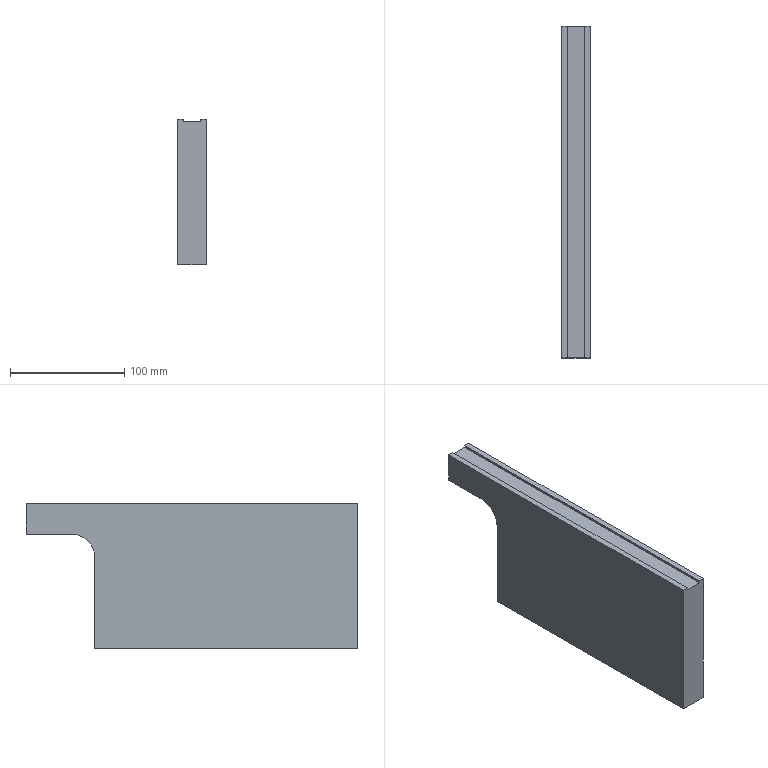Part | STEP file | Tube necking machine_id718_x_t | 1 solid | 13 faces | box 25 x 290 x 127 mm | volume 764196 mm3 | plane 12 | cylinder 1 | commonest cylinder face diameters 40 x1
STEP:
#1=CARTESIAN_POINT('',(0.,0.,0.));
#2=DIRECTION('',(0.,0.,1.));
#3=DIRECTION('',(1.,0.,0.));
#4=AXIS2_PLACEMENT_3D('',#1,#2,#3);
#5=CARTESIAN_POINT('',(192.5,-276.,145.));
#6=VERTEX_POINT('',#5);
#7=CARTESIAN_POINT('',(192.5,-276.,147.));
#8=VERTEX_POINT('',#7);
#9=CARTESIAN_POINT('',(192.5,-276.,146.181));
#10=DIRECTION('',(0.,0.,1.));
#11=VECTOR('',#10,1.);
#12=LINE('',#9,#11);
#13=CARTESIAN_POINT('',(197.5,-276.,110.));
#14=DIRECTION('',(0.,1.,0.));
#15=DIRECTION('',(0.,0.,1.));
#16=AXIS2_PLACEMENT_3D('',#13,#14,#15);
#17=PLANE('',#16);
#18=CARTESIAN_POINT('',(36.181,-5.));
#19=DIRECTION('',(1.,0.));
#20=VECTOR('',#19,1.);
#21=LINE('',#18,#20);
#22=(GEOMETRIC_REPRESENTATION_CONTEXT(2)PARAMETRIC_REPRESENTATION_CONTEXT()REPRESENTATION_CONTEXT('',''));
#23=DEFINITIONAL_REPRESENTATION('',(#21),#22);
#24=PCURVE('',#17,#23);
#25=CARTESIAN_POINT('',(192.5,795.73,146.181));
#26=DIRECTION('',(1.,0.,0.));
#27=DIRECTION('',(0.,0.,1.));
#28=AXIS2_PLACEMENT_3D('',#25,#26,#27);
#29=PLANE('',#28);
#30=CARTESIAN_POINT('',(0.,1071.73));
#31=DIRECTION('',(1.,0.));
#32=VECTOR('',#31,1.);
#33=LINE('',#30,#32);
#34=(GEOMETRIC_REPRESENTATION_CONTEXT(2)PARAMETRIC_REPRESENTATION_CONTEXT()REPRESENTATION_CONTEXT('',''));
#35=DEFINITIONAL_REPRESENTATION('',(#33),#34);
#36=PCURVE('',#29,#35);
#37=SURFACE_CURVE('',#12,(#24,#36),.PCURVE_S1.);
#38=EDGE_CURVE('',#6,#8,#37,.T.);
#39=ORIENTED_EDGE('',*,*,#38,.F.);
#40=CARTESIAN_POINT('',(177.5,-276.,145.));
#41=VERTEX_POINT('',#40);
#42=CARTESIAN_POINT('',(192.5,-276.,145.));
#43=DIRECTION('',(1.,0.,0.));
#44=VECTOR('',#43,1.);
#45=LINE('',#42,#44);
#46=CARTESIAN_POINT('',(35.,-5.));
#47=DIRECTION('',(0.,1.));
#48=VECTOR('',#47,1.);
#49=LINE('',#46,#48);
#50=(GEOMETRIC_REPRESENTATION_CONTEXT(2)PARAMETRIC_REPRESENTATION_CONTEXT()REPRESENTATION_CONTEXT('',''));
#51=DEFINITIONAL_REPRESENTATION('',(#49),#50);
#52=PCURVE('',#17,#51);
#53=CARTESIAN_POINT('',(192.5,795.73,145.));
#54=DIRECTION('',(0.,0.,-1.));
#55=DIRECTION('',(0.,-1.,0.));
#56=AXIS2_PLACEMENT_3D('',#53,#54,#55);
#57=PLANE('',#56);
#58=CARTESIAN_POINT('',(1071.73,0.));
#59=DIRECTION('',(0.,-1.));
#60=VECTOR('',#59,1.);
#61=LINE('',#58,#60);
#62=(GEOMETRIC_REPRESENTATION_CONTEXT(2)PARAMETRIC_REPRESENTATION_CONTEXT()REPRESENTATION_CONTEXT('',''));
#63=DEFINITIONAL_REPRESENTATION('',(#61),#62);
#64=PCURVE('',#57,#63);
#65=SURFACE_CURVE('',#45,(#52,#64),.PCURVE_S1.);
#66=EDGE_CURVE('',#41,#6,#65,.T.);
#67=ORIENTED_EDGE('',*,*,#66,.F.);
#68=CARTESIAN_POINT('',(177.5,-276.,147.));
#69=VERTEX_POINT('',#68);
#70=CARTESIAN_POINT('',(177.5,-276.,145.));
#71=DIRECTION('',(0.,0.,-1.));
#72=VECTOR('',#71,1.);
#73=LINE('',#70,#72);
#74=CARTESIAN_POINT('',(35.,-20.));
#75=DIRECTION('',(-1.,0.));
#76=VECTOR('',#75,1.);
#77=LINE('',#74,#76);
#78=(GEOMETRIC_REPRESENTATION_CONTEXT(2)PARAMETRIC_REPRESENTATION_CONTEXT()REPRESENTATION_CONTEXT('',''));
#79=DEFINITIONAL_REPRESENTATION('',(#77),#78);
#80=PCURVE('',#17,#79);
#81=CARTESIAN_POINT('',(177.5,795.73,145.));
#82=DIRECTION('',(-1.,0.,0.));
#83=DIRECTION('',(0.,0.,-1.));
#84=AXIS2_PLACEMENT_3D('',#81,#82,#83);
#85=PLANE('',#84);
#86=CARTESIAN_POINT('',(0.,1071.73));
#87=DIRECTION('',(1.,0.));
#88=VECTOR('',#87,1.);
#89=LINE('',#86,#88);
#90=(GEOMETRIC_REPRESENTATION_CONTEXT(2)PARAMETRIC_REPRESENTATION_CONTEXT()REPRESENTATION_CONTEXT('',''));
#91=DEFINITIONAL_REPRESENTATION('',(#89),#90);
#92=PCURVE('',#85,#91);
#93=SURFACE_CURVE('',#73,(#80,#92),.PCURVE_S1.);
#94=EDGE_CURVE('',#69,#41,#93,.T.);
#95=ORIENTED_EDGE('',*,*,#94,.F.);
#96=CARTESIAN_POINT('',(172.5,-276.,147.));
#97=VERTEX_POINT('',#96);
#98=CARTESIAN_POINT('',(197.5,-276.,147.));
#99=DIRECTION('',(1.,0.,0.));
#100=VECTOR('',#99,1.);
#101=LINE('',#98,#100);
#102=CARTESIAN_POINT('',(37.,0.));
#103=DIRECTION('',(0.,1.));
#104=VECTOR('',#103,1.);
#105=LINE('',#102,#104);
#106=(GEOMETRIC_REPRESENTATION_CONTEXT(2)PARAMETRIC_REPRESENTATION_CONTEXT()REPRESENTATION_CONTEXT('',''));
#107=DEFINITIONAL_REPRESENTATION('',(#105),#106);
#108=PCURVE('',#17,#107);
#109=CARTESIAN_POINT('',(0.,0.,147.));
#110=DIRECTION('',(0.,0.,1.));
#111=DIRECTION('',(-1.,0.,0.));
#112=AXIS2_PLACEMENT_3D('',#109,#110,#111);
#113=PLANE('',#112);
#114=CARTESIAN_POINT('',(-197.5,276.));
#115=DIRECTION('',(-1.,0.));
#116=VECTOR('',#115,1.);
#117=LINE('',#114,#116);
#118=(GEOMETRIC_REPRESENTATION_CONTEXT(2)PARAMETRIC_REPRESENTATION_CONTEXT()REPRESENTATION_CONTEXT('',''));
#119=DEFINITIONAL_REPRESENTATION('',(#117),#118);
#120=PCURVE('',#113,#119);
#121=SURFACE_CURVE('',#101,(#108,#120),.PCURVE_S1.);
#122=EDGE_CURVE('',#97,#69,#121,.T.);
#123=ORIENTED_EDGE('',*,*,#122,.F.);
#124=CARTESIAN_POINT('',(172.5,-276.,20.));
#125=VERTEX_POINT('',#124);
#126=CARTESIAN_POINT('',(172.5,-276.,110.));
#127=DIRECTION('',(0.,0.,1.));
#128=VECTOR('',#127,1.);
#129=LINE('',#126,#128);
#130=CARTESIAN_POINT('',(0.,-25.));
#131=DIRECTION('',(1.,0.));
#132=VECTOR('',#131,1.);
#133=LINE('',#130,#132);
#134=(GEOMETRIC_REPRESENTATION_CONTEXT(2)PARAMETRIC_REPRESENTATION_CONTEXT()REPRESENTATION_CONTEXT('',''));
#135=DEFINITIONAL_REPRESENTATION('',(#133),#134);
#136=PCURVE('',#17,#135);
#137=CARTESIAN_POINT('',(172.5,-276.,110.));
#138=DIRECTION('',(1.,0.,0.));
#139=DIRECTION('',(0.,0.,1.));
#140=AXIS2_PLACEMENT_3D('',#137,#138,#139);
#141=PLANE('',#140);
#142=CARTESIAN_POINT('',(0.,0.));
#143=DIRECTION('',(1.,0.));
#144=VECTOR('',#143,1.);
#145=LINE('',#142,#144);
#146=(GEOMETRIC_REPRESENTATION_CONTEXT(2)PARAMETRIC_REPRESENTATION_CONTEXT()REPRESENTATION_CONTEXT('',''));
#147=DEFINITIONAL_REPRESENTATION('',(#145),#146);
#148=PCURVE('',#141,#147);
#149=SURFACE_CURVE('',#129,(#136,#148),.PCURVE_S1.);
#150=EDGE_CURVE('',#125,#97,#149,.T.);
#151=ORIENTED_EDGE('',*,*,#150,.F.);
#152=CARTESIAN_POINT('',(197.5,-276.,20.));
#153=VERTEX_POINT('',#152);
#154=CARTESIAN_POINT('',(197.5,-276.,20.));
#155=DIRECTION('',(1.,0.,0.));
#156=VECTOR('',#155,1.);
#157=LINE('',#154,#156);
#158=CARTESIAN_POINT('',(-90.,0.));
#159=DIRECTION('',(0.,1.));
#160=VECTOR('',#159,1.);
#161=LINE('',#158,#160);
#162=(GEOMETRIC_REPRESENTATION_CONTEXT(2)PARAMETRIC_REPRESENTATION_CONTEXT()REPRESENTATION_CONTEXT('',''));
#163=DEFINITIONAL_REPRESENTATION('',(#161),#162);
#164=PCURVE('',#17,#163);
#165=CARTESIAN_POINT('',(0.,0.,20.));
#166=DIRECTION('',(0.,0.,1.));
#167=DIRECTION('',(-1.,0.,0.));
#168=AXIS2_PLACEMENT_3D('',#165,#166,#167);
#169=PLANE('',#168);
#170=CARTESIAN_POINT('',(-197.5,276.));
#171=DIRECTION('',(-1.,0.));
#172=VECTOR('',#171,1.);
#173=LINE('',#170,#172);
#174=(GEOMETRIC_REPRESENTATION_CONTEXT(2)PARAMETRIC_REPRESENTATION_CONTEXT()REPRESENTATION_CONTEXT('',''));
#175=DEFINITIONAL_REPRESENTATION('',(#173),#174);
#176=PCURVE('',#169,#175);
#177=SURFACE_CURVE('',#157,(#164,#176),.PCURVE_S1.);
#178=EDGE_CURVE('',#125,#153,#177,.T.);
#179=ORIENTED_EDGE('',*,*,#178,.T.);
#180=CARTESIAN_POINT('',(197.5,-276.,147.));
#181=VERTEX_POINT('',#180);
#182=CARTESIAN_POINT('',(197.5,-276.,110.));
#183=DIRECTION('',(0.,0.,1.));
#184=VECTOR('',#183,1.);
#185=LINE('',#182,#184);
#186=CARTESIAN_POINT('',(0.,0.));
#187=DIRECTION('',(1.,0.));
#188=VECTOR('',#187,1.);
#189=LINE('',#186,#188);
#190=(GEOMETRIC_REPRESENTATION_CONTEXT(2)PARAMETRIC_REPRESENTATION_CONTEXT()REPRESENTATION_CONTEXT('',''));
#191=DEFINITIONAL_REPRESENTATION('',(#189),#190);
#192=PCURVE('',#17,#191);
#193=CARTESIAN_POINT('',(197.5,-46.,110.));
#194=DIRECTION('',(-1.,0.,0.));
#195=DIRECTION('',(0.,0.,-1.));
#196=AXIS2_PLACEMENT_3D('',#193,#194,#195);
#197=PLANE('',#196);
#198=CARTESIAN_POINT('',(0.,230.));
#199=DIRECTION('',(-1.,0.));
#200=VECTOR('',#199,1.);
#201=LINE('',#198,#200);
#202=(GEOMETRIC_REPRESENTATION_CONTEXT(2)PARAMETRIC_REPRESENTATION_CONTEXT()REPRESENTATION_CONTEXT('',''));
#203=DEFINITIONAL_REPRESENTATION('',(#201),#202);
#204=PCURVE('',#197,#203);
#205=SURFACE_CURVE('',#185,(#192,#204),.PCURVE_S1.);
#206=EDGE_CURVE('',#153,#181,#205,.T.);
#207=ORIENTED_EDGE('',*,*,#206,.T.);
#208=CARTESIAN_POINT('',(197.5,-276.,147.));
#209=DIRECTION('',(1.,0.,0.));
#210=VECTOR('',#209,1.);
#211=LINE('',#208,#210);
#212=CARTESIAN_POINT('',(37.,0.));
#213=DIRECTION('',(0.,1.));
#214=VECTOR('',#213,1.);
#215=LINE('',#212,#214);
#216=(GEOMETRIC_REPRESENTATION_CONTEXT(2)PARAMETRIC_REPRESENTATION_CONTEXT()REPRESENTATION_CONTEXT('',''));
#217=DEFINITIONAL_REPRESENTATION('',(#215),#216);
#218=PCURVE('',#17,#217);
#219=CARTESIAN_POINT('',(0.,0.,147.));
#220=DIRECTION('',(0.,0.,1.));
#221=DIRECTION('',(-1.,0.,0.));
#222=AXIS2_PLACEMENT_3D('',#219,#220,#221);
#223=PLANE('',#222);
#224=CARTESIAN_POINT('',(-197.5,276.));
#225=DIRECTION('',(-1.,0.));
#226=VECTOR('',#225,1.);
#227=LINE('',#224,#226);
#228=(GEOMETRIC_REPRESENTATION_CONTEXT(2)PARAMETRIC_REPRESENTATION_CONTEXT()REPRESENTATION_CONTEXT('',''));
#229=DEFINITIONAL_REPRESENTATION('',(#227),#228);
#230=PCURVE('',#223,#229);
#231=SURFACE_CURVE('',#211,(#218,#230),.PCURVE_S1.);
#232=EDGE_CURVE('',#8,#181,#231,.T.);
#233=ORIENTED_EDGE('',*,*,#232,.F.);
#234=EDGE_LOOP('',(#39,#67,#95,#123,#151,#179,#207,#233));
#235=FACE_BOUND('',#234,.T.);
#236=ADVANCED_FACE('',(#235),#17,.F.);
#237=CARTESIAN_POINT('',(177.5,14.,147.));
#238=VERTEX_POINT('',#237);
#239=CARTESIAN_POINT('',(177.5,0.,147.));
#240=DIRECTION('',(0.,-1.,0.));
#241=VECTOR('',#240,1.);
#242=LINE('',#239,#241);
#243=CARTESIAN_POINT('',(-177.5,0.));
#244=DIRECTION('',(0.,1.));
#245=VECTOR('',#244,1.);
#246=LINE('',#243,#245);
#247=(GEOMETRIC_REPRESENTATION_CONTEXT(2)PARAMETRIC_REPRESENTATION_CONTEXT()REPRESENTATION_CONTEXT('',''));
#248=DEFINITIONAL_REPRESENTATION('',(#246),#247);
#249=PCURVE('',#113,#248);
#250=CARTESIAN_POINT('',(-2.,795.73));
#251=DIRECTION('',(0.,1.));
#252=VECTOR('',#251,1.);
#253=LINE('',#250,#252);
#254=(GEOMETRIC_REPRESENTATION_CONTEXT(2)PARAMETRIC_REPRESENTATION_CONTEXT()REPRESENTATION_CONTEXT('',''));
#255=DEFINITIONAL_REPRESENTATION('',(#253),#254);
#256=PCURVE('',#85,#255);
#257=SURFACE_CURVE('',#242,(#249,#256),.PCURVE_S1.);
#258=EDGE_CURVE('',#238,#69,#257,.T.);
#259=ORIENTED_EDGE('',*,*,#258,.F.);
#260=CARTESIAN_POINT('',(172.5,14.,147.));
#261=VERTEX_POINT('',#260);
#262=CARTESIAN_POINT('',(197.5,14.,147.));
#263=DIRECTION('',(1.,0.,0.));
#264=VECTOR('',#263,1.);
#265=LINE('',#262,#264);
#266=CARTESIAN_POINT('',(-197.5,-14.));
#267=DIRECTION('',(-1.,0.));
#268=VECTOR('',#267,1.);
#269=LINE('',#266,#268);
#270=(GEOMETRIC_REPRESENTATION_CONTEXT(2)PARAMETRIC_REPRESENTATION_CONTEXT()REPRESENTATION_CONTEXT('',''));
#271=DEFINITIONAL_REPRESENTATION('',(#269),#270);
#272=PCURVE('',#113,#271);
#273=CARTESIAN_POINT('',(197.5,14.,151.));
#274=DIRECTION('',(0.,1.,0.));
#275=DIRECTION('',(-1.,0.,0.));
#276=AXIS2_PLACEMENT_3D('',#273,#274,#275);
#277=PLANE('',#276);
#278=CARTESIAN_POINT('',(0.,-4.));
#279=DIRECTION('',(-1.,0.));
#280=VECTOR('',#279,1.);
#281=LINE('',#278,#280);
#282=(GEOMETRIC_REPRESENTATION_CONTEXT(2)PARAMETRIC_REPRESENTATION_CONTEXT()REPRESENTATION_CONTEXT('',''));
#283=DEFINITIONAL_REPRESENTATION('',(#281),#282);
#284=PCURVE('',#277,#283);
#285=SURFACE_CURVE('',#265,(#272,#284),.PCURVE_S1.);
#286=EDGE_CURVE('',#261,#238,#285,.T.);
#287=ORIENTED_EDGE('',*,*,#286,.F.);
#288=CARTESIAN_POINT('',(172.5,-276.,147.));
#289=DIRECTION('',(0.,-1.,0.));
#290=VECTOR('',#289,1.);
#291=LINE('',#288,#290);
#292=CARTESIAN_POINT('',(-172.5,276.));
#293=DIRECTION('',(0.,1.));
#294=VECTOR('',#293,1.);
#295=LINE('',#292,#294);
#296=(GEOMETRIC_REPRESENTATION_CONTEXT(2)PARAMETRIC_REPRESENTATION_CONTEXT()REPRESENTATION_CONTEXT('',''));
#297=DEFINITIONAL_REPRESENTATION('',(#295),#296);
#298=PCURVE('',#113,#297);
#299=CARTESIAN_POINT('',(37.,0.));
#300=DIRECTION('',(0.,1.));
#301=VECTOR('',#300,1.);
#302=LINE('',#299,#301);
#303=(GEOMETRIC_REPRESENTATION_CONTEXT(2)PARAMETRIC_REPRESENTATION_CONTEXT()REPRESENTATION_CONTEXT('',''));
#304=DEFINITIONAL_REPRESENTATION('',(#302),#303);
#305=PCURVE('',#141,#304);
#306=SURFACE_CURVE('',#291,(#298,#305),.PCURVE_S1.);
#307=EDGE_CURVE('',#261,#97,#306,.T.);
#308=ORIENTED_EDGE('',*,*,#307,.T.);
#309=ORIENTED_EDGE('',*,*,#122,.T.);
#310=EDGE_LOOP('',(#259,#287,#308,#309));
#311=FACE_BOUND('',#310,.T.);
#312=ADVANCED_FACE('',(#311),#113,.T.);
#313=ORIENTED_EDGE('',*,*,#206,.F.);
#314=CARTESIAN_POINT('',(197.5,-46.,20.));
#315=VERTEX_POINT('',#314);
#316=CARTESIAN_POINT('',(197.5,-46.,20.));
#317=DIRECTION('',(0.,1.,0.));
#318=VECTOR('',#317,1.);
#319=LINE('',#316,#318);
#320=CARTESIAN_POINT('',(90.,0.));
#321=DIRECTION('',(0.,-1.));
#322=VECTOR('',#321,1.);
#323=LINE('',#320,#322);
#324=(GEOMETRIC_REPRESENTATION_CONTEXT(2)PARAMETRIC_REPRESENTATION_CONTEXT()REPRESENTATION_CONTEXT('',''));
#325=DEFINITIONAL_REPRESENTATION('',(#323),#324);
#326=PCURVE('',#197,#325);
#327=CARTESIAN_POINT('',(-197.5,46.));
#328=DIRECTION('',(0.,-1.));
#329=VECTOR('',#328,1.);
#330=LINE('',#327,#329);
#331=(GEOMETRIC_REPRESENTATION_CONTEXT(2)PARAMETRIC_REPRESENTATION_CONTEXT()REPRESENTATION_CONTEXT('',''));
#332=DEFINITIONAL_REPRESENTATION('',(#330),#331);
#333=PCURVE('',#169,#332);
#334=SURFACE_CURVE('',#319,(#326,#333),.PCURVE_S1.);
#335=EDGE_CURVE('',#153,#315,#334,.T.);
#336=ORIENTED_EDGE('',*,*,#335,.T.);
#337=CARTESIAN_POINT('',(197.5,-46.,100.));
#338=VERTEX_POINT('',#337);
#339=CARTESIAN_POINT('',(197.5,-46.,110.));
#340=DIRECTION('',(0.,0.,1.));
#341=VECTOR('',#340,1.);
#342=LINE('',#339,#341);
#343=CARTESIAN_POINT('',(0.,0.));
#344=DIRECTION('',(-1.,0.));
#345=VECTOR('',#344,1.);
#346=LINE('',#343,#345);
#347=(GEOMETRIC_REPRESENTATION_CONTEXT(2)PARAMETRIC_REPRESENTATION_CONTEXT()REPRESENTATION_CONTEXT('',''));
#348=DEFINITIONAL_REPRESENTATION('',(#346),#347);
#349=PCURVE('',#197,#348);
#350=CARTESIAN_POINT('',(172.5,-46.,110.));
#351=DIRECTION('',(0.,-1.,0.));
#352=DIRECTION('',(0.,0.,-1.));
#353=AXIS2_PLACEMENT_3D('',#350,#351,#352);
#354=PLANE('',#353);
#355=CARTESIAN_POINT('',(0.,25.));
#356=DIRECTION('',(-1.,0.));
#357=VECTOR('',#356,1.);
#358=LINE('',#355,#357);
#359=(GEOMETRIC_REPRESENTATION_CONTEXT(2)PARAMETRIC_REPRESENTATION_CONTEXT()REPRESENTATION_CONTEXT('',''));
#360=DEFINITIONAL_REPRESENTATION('',(#358),#359);
#361=PCURVE('',#354,#360);
#362=SURFACE_CURVE('',#342,(#349,#361),.PCURVE_S1.);
#363=EDGE_CURVE('',#315,#338,#362,.T.);
#364=ORIENTED_EDGE('',*,*,#363,.T.);
#365=CARTESIAN_POINT('',(197.5,-26.,120.));
#366=VERTEX_POINT('',#365);
#367=CARTESIAN_POINT('',(197.5,-26.,100.));
#368=DIRECTION('',(-1.,0.,0.));
#369=DIRECTION('',(0.,0.,-1.));
#370=AXIS2_PLACEMENT_3D('',#367,#368,#369);
#371=CIRCLE('',#370,20.);
#372=CARTESIAN_POINT('',(10.,-20.));
#373=DIRECTION('',(1.,0.));
#374=AXIS2_PLACEMENT_2D('',#372,#373);
#375=CIRCLE('',#374,20.);
#376=(GEOMETRIC_REPRESENTATION_CONTEXT(2)PARAMETRIC_REPRESENTATION_CONTEXT()REPRESENTATION_CONTEXT('',''));
#377=DEFINITIONAL_REPRESENTATION('',(#375),#376);
#378=PCURVE('',#197,#377);
#379=CARTESIAN_POINT('',(172.5,-26.,100.));
#380=DIRECTION('',(1.,0.,0.));
#381=DIRECTION('',(0.,0.,1.));
#382=AXIS2_PLACEMENT_3D('',#379,#380,#381);
#383=CYLINDRICAL_SURFACE('',#382,20.);
#384=CARTESIAN_POINT('',(3.142,25.));
#385=DIRECTION('',(-1.,0.));
#386=VECTOR('',#385,1.);
#387=LINE('',#384,#386);
#388=(GEOMETRIC_REPRESENTATION_CONTEXT(2)PARAMETRIC_REPRESENTATION_CONTEXT()REPRESENTATION_CONTEXT('',''));
#389=DEFINITIONAL_REPRESENTATION('',(#387),#388);
#390=PCURVE('',#383,#389);
#391=SURFACE_CURVE('',#371,(#378,#390),.PCURVE_S1.);
#392=EDGE_CURVE('',#338,#366,#391,.T.);
#393=ORIENTED_EDGE('',*,*,#392,.T.);
#394=CARTESIAN_POINT('',(197.5,14.,120.));
#395=VERTEX_POINT('',#394);
#396=CARTESIAN_POINT('',(197.5,0.,120.));
#397=DIRECTION('',(0.,1.,0.));
#398=VECTOR('',#397,1.);
#399=LINE('',#396,#398);
#400=CARTESIAN_POINT('',(-10.,-46.));
#401=DIRECTION('',(0.,-1.));
#402=VECTOR('',#401,1.);
#403=LINE('',#400,#402);
#404=(GEOMETRIC_REPRESENTATION_CONTEXT(2)PARAMETRIC_REPRESENTATION_CONTEXT()REPRESENTATION_CONTEXT('',''));
#405=DEFINITIONAL_REPRESENTATION('',(#403),#404);
#406=PCURVE('',#197,#405);
#407=CARTESIAN_POINT('',(0.,0.,120.));
#408=DIRECTION('',(0.,0.,1.));
#409=DIRECTION('',(-1.,0.,0.));
#410=AXIS2_PLACEMENT_3D('',#407,#408,#409);
#411=PLANE('',#410);
#412=CARTESIAN_POINT('',(-197.5,0.));
#413=DIRECTION('',(0.,-1.));
#414=VECTOR('',#413,1.);
#415=LINE('',#412,#414);
#416=(GEOMETRIC_REPRESENTATION_CONTEXT(2)PARAMETRIC_REPRESENTATION_CONTEXT()REPRESENTATION_CONTEXT('',''));
#417=DEFINITIONAL_REPRESENTATION('',(#415),#416);
#418=PCURVE('',#411,#417);
#419=SURFACE_CURVE('',#399,(#406,#418),.PCURVE_S1.);
#420=EDGE_CURVE('',#366,#395,#419,.T.);
#421=ORIENTED_EDGE('',*,*,#420,.T.);
#422=CARTESIAN_POINT('',(197.5,14.,147.));
#423=VERTEX_POINT('',#422);
#424=CARTESIAN_POINT('',(197.5,14.,151.));
#425=DIRECTION('',(0.,0.,1.));
#426=VECTOR('',#425,1.);
#427=LINE('',#424,#426);
#428=CARTESIAN_POINT('',(-41.,-60.));
#429=DIRECTION('',(-1.,0.));
#430=VECTOR('',#429,1.);
#431=LINE('',#428,#430);
#432=(GEOMETRIC_REPRESENTATION_CONTEXT(2)PARAMETRIC_REPRESENTATION_CONTEXT()REPRESENTATION_CONTEXT('',''));
#433=DEFINITIONAL_REPRESENTATION('',(#431),#432);
#434=PCURVE('',#197,#433);
#435=CARTESIAN_POINT('',(0.,0.));
#436=DIRECTION('',(0.,1.));
#437=VECTOR('',#436,1.);
#438=LINE('',#435,#437);
#439=(GEOMETRIC_REPRESENTATION_CONTEXT(2)PARAMETRIC_REPRESENTATION_CONTEXT()REPRESENTATION_CONTEXT('',''));
#440=DEFINITIONAL_REPRESENTATION('',(#438),#439);
#441=PCURVE('',#277,#440);
#442=SURFACE_CURVE('',#427,(#434,#441),.PCURVE_S1.);
#443=EDGE_CURVE('',#395,#423,#442,.T.);
#444=ORIENTED_EDGE('',*,*,#443,.T.);
#445=CARTESIAN_POINT('',(197.5,-46.,147.));
#446=DIRECTION('',(0.,1.,0.));
#447=VECTOR('',#446,1.);
#448=LINE('',#445,#447);
#449=CARTESIAN_POINT('',(-37.,0.));
#450=DIRECTION('',(0.,-1.));
#451=VECTOR('',#450,1.);
#452=LINE('',#449,#451);
#453=(GEOMETRIC_REPRESENTATION_CONTEXT(2)PARAMETRIC_REPRESENTATION_CONTEXT()REPRESENTATION_CONTEXT('',''));
#454=DEFINITIONAL_REPRESENTATION('',(#452),#453);
#455=PCURVE('',#197,#454);
#456=CARTESIAN_POINT('',(-197.5,46.));
#457=DIRECTION('',(0.,-1.));
#458=VECTOR('',#457,1.);
#459=LINE('',#456,#458);
#460=(GEOMETRIC_REPRESENTATION_CONTEXT(2)PARAMETRIC_REPRESENTATION_CONTEXT()REPRESENTATION_CONTEXT('',''));
#461=DEFINITIONAL_REPRESENTATION('',(#459),#460);
#462=PCURVE('',#223,#461);
#463=SURFACE_CURVE('',#448,(#455,#462),.PCURVE_S1.);
#464=EDGE_CURVE('',#181,#423,#463,.T.);
#465=ORIENTED_EDGE('',*,*,#464,.F.);
#466=EDGE_LOOP('',(#313,#336,#364,#393,#421,#444,#465));
#467=FACE_BOUND('',#466,.T.);
#468=ADVANCED_FACE('',(#467),#197,.F.);
#469=ORIENTED_EDGE('',*,*,#307,.F.);
#470=CARTESIAN_POINT('',(172.5,14.,120.));
#471=VERTEX_POINT('',#470);
#472=CARTESIAN_POINT('',(172.5,14.,110.));
#473=DIRECTION('',(0.,0.,1.));
#474=VECTOR('',#473,1.);
#475=LINE('',#472,#474);
#476=CARTESIAN_POINT('',(0.,-290.));
#477=DIRECTION('',(1.,0.));
#478=VECTOR('',#477,1.);
#479=LINE('',#476,#478);
#480=(GEOMETRIC_REPRESENTATION_CONTEXT(2)PARAMETRIC_REPRESENTATION_CONTEXT()REPRESENTATION_CONTEXT('',''));
#481=DEFINITIONAL_REPRESENTATION('',(#479),#480);
#482=PCURVE('',#141,#481);
#483=CARTESIAN_POINT('',(25.,-41.));
#484=DIRECTION('',(0.,1.));
#485=VECTOR('',#484,1.);
#486=LINE('',#483,#485);
#487=(GEOMETRIC_REPRESENTATION_CONTEXT(2)PARAMETRIC_REPRESENTATION_CONTEXT()REPRESENTATION_CONTEXT('',''));
#488=DEFINITIONAL_REPRESENTATION('',(#486),#487);
#489=PCURVE('',#277,#488);
#490=SURFACE_CURVE('',#475,(#482,#489),.PCURVE_S1.);
#491=EDGE_CURVE('',#471,#261,#490,.T.);
#492=ORIENTED_EDGE('',*,*,#491,.F.);
#493=CARTESIAN_POINT('',(172.5,-26.,120.));
#494=VERTEX_POINT('',#493);
#495=CARTESIAN_POINT('',(172.5,-276.,120.));
#496=DIRECTION('',(0.,1.,0.));
#497=VECTOR('',#496,1.);
#498=LINE('',#495,#497);
#499=CARTESIAN_POINT('',(10.,0.));
#500=DIRECTION('',(0.,-1.));
#501=VECTOR('',#500,1.);
#502=LINE('',#499,#501);
#503=(GEOMETRIC_REPRESENTATION_CONTEXT(2)PARAMETRIC_REPRESENTATION_CONTEXT()REPRESENTATION_CONTEXT('',''));
#504=DEFINITIONAL_REPRESENTATION('',(#502),#503);
#505=PCURVE('',#141,#504);
#506=CARTESIAN_POINT('',(-172.5,276.));
#507=DIRECTION('',(0.,-1.));
#508=VECTOR('',#507,1.);
#509=LINE('',#506,#508);
#510=(GEOMETRIC_REPRESENTATION_CONTEXT(2)PARAMETRIC_REPRESENTATION_CONTEXT()REPRESENTATION_CONTEXT('',''));
#511=DEFINITIONAL_REPRESENTATION('',(#509),#510);
#512=PCURVE('',#411,#511);
#513=SURFACE_CURVE('',#498,(#505,#512),.PCURVE_S1.);
#514=EDGE_CURVE('',#494,#471,#513,.T.);
#515=ORIENTED_EDGE('',*,*,#514,.F.);
#516=CARTESIAN_POINT('',(172.5,-46.,100.));
#517=VERTEX_POINT('',#516);
#518=CARTESIAN_POINT('',(172.5,-26.,100.));
#519=DIRECTION('',(1.,0.,0.));
#520=DIRECTION('',(0.,0.,1.));
#521=AXIS2_PLACEMENT_3D('',#518,#519,#520);
#522=CIRCLE('',#521,20.);
#523=CARTESIAN_POINT('',(-10.,-250.));
#524=DIRECTION('',(1.,0.));
#525=AXIS2_PLACEMENT_2D('',#523,#524);
#526=CIRCLE('',#525,20.);
#527=(GEOMETRIC_REPRESENTATION_CONTEXT(2)PARAMETRIC_REPRESENTATION_CONTEXT()REPRESENTATION_CONTEXT('',''));
#528=DEFINITIONAL_REPRESENTATION('',(#526),#527);
#529=PCURVE('',#141,#528);
#530=CARTESIAN_POINT('',(0.,0.));
#531=DIRECTION('',(1.,0.));
#532=VECTOR('',#531,1.);
#533=LINE('',#530,#532);
#534=(GEOMETRIC_REPRESENTATION_CONTEXT(2)PARAMETRIC_REPRESENTATION_CONTEXT()REPRESENTATION_CONTEXT('',''));
#535=DEFINITIONAL_REPRESENTATION('',(#533),#534);
#536=PCURVE('',#383,#535);
#537=SURFACE_CURVE('',#522,(#529,#536),.PCURVE_S1.);
#538=EDGE_CURVE('',#494,#517,#537,.T.);
#539=ORIENTED_EDGE('',*,*,#538,.T.);
#540=CARTESIAN_POINT('',(172.5,-46.,20.));
#541=VERTEX_POINT('',#540);
#542=CARTESIAN_POINT('',(172.5,-46.,110.));
#543=DIRECTION('',(0.,0.,1.));
#544=VECTOR('',#543,1.);
#545=LINE('',#542,#544);
#546=CARTESIAN_POINT('',(0.,-230.));
#547=DIRECTION('',(1.,0.));
#548=VECTOR('',#547,1.);
#549=LINE('',#546,#548);
#550=(GEOMETRIC_REPRESENTATION_CONTEXT(2)PARAMETRIC_REPRESENTATION_CONTEXT()REPRESENTATION_CONTEXT('',''));
#551=DEFINITIONAL_REPRESENTATION('',(#549),#550);
#552=PCURVE('',#141,#551);
#553=CARTESIAN_POINT('',(0.,0.));
#554=DIRECTION('',(-1.,0.));
#555=VECTOR('',#554,1.);
#556=LINE('',#553,#555);
#557=(GEOMETRIC_REPRESENTATION_CONTEXT(2)PARAMETRIC_REPRESENTATION_CONTEXT()REPRESENTATION_CONTEXT('',''));
#558=DEFINITIONAL_REPRESENTATION('',(#556),#557);
#559=PCURVE('',#354,#558);
#560=SURFACE_CURVE('',#545,(#552,#559),.PCURVE_S1.);
#561=EDGE_CURVE('',#541,#517,#560,.T.);
#562=ORIENTED_EDGE('',*,*,#561,.F.);
#563=CARTESIAN_POINT('',(172.5,-276.,20.));
#564=DIRECTION('',(0.,-1.,0.));
#565=VECTOR('',#564,1.);
#566=LINE('',#563,#565);
#567=CARTESIAN_POINT('',(-90.,0.));
#568=DIRECTION('',(0.,1.));
#569=VECTOR('',#568,1.);
#570=LINE('',#567,#569);
#571=(GEOMETRIC_REPRESENTATION_CONTEXT(2)PARAMETRIC_REPRESENTATION_CONTEXT()REPRESENTATION_CONTEXT('',''));
#572=DEFINITIONAL_REPRESENTATION('',(#570),#571);
#573=PCURVE('',#141,#572);
#574=CARTESIAN_POINT('',(-172.5,276.));
#575=DIRECTION('',(0.,1.));
#576=VECTOR('',#575,1.);
#577=LINE('',#574,#576);
#578=(GEOMETRIC_REPRESENTATION_CONTEXT(2)PARAMETRIC_REPRESENTATION_CONTEXT()REPRESENTATION_CONTEXT('',''));
#579=DEFINITIONAL_REPRESENTATION('',(#577),#578);
#580=PCURVE('',#169,#579);
#581=SURFACE_CURVE('',#566,(#573,#580),.PCURVE_S1.);
#582=EDGE_CURVE('',#541,#125,#581,.T.);
#583=ORIENTED_EDGE('',*,*,#582,.T.);
#584=ORIENTED_EDGE('',*,*,#150,.T.);
#585=EDGE_LOOP('',(#469,#492,#515,#539,#562,#583,#584));
#586=FACE_BOUND('',#585,.T.);
#587=ADVANCED_FACE('',(#586),#141,.F.);
#588=ORIENTED_EDGE('',*,*,#363,.F.);
#589=CARTESIAN_POINT('',(172.5,-46.,20.));
#590=DIRECTION('',(-1.,0.,0.));
#591=VECTOR('',#590,1.);
#592=LINE('',#589,#591);
#593=CARTESIAN_POINT('',(90.,0.));
#594=DIRECTION('',(0.,-1.));
#595=VECTOR('',#594,1.);
#596=LINE('',#593,#595);
#597=(GEOMETRIC_REPRESENTATION_CONTEXT(2)PARAMETRIC_REPRESENTATION_CONTEXT()REPRESENTATION_CONTEXT('',''));
#598=DEFINITIONAL_REPRESENTATION('',(#596),#597);
#599=PCURVE('',#354,#598);
#600=CARTESIAN_POINT('',(-172.5,46.));
#601=DIRECTION('',(1.,0.));
#602=VECTOR('',#601,1.);
#603=LINE('',#600,#602);
#604=(GEOMETRIC_REPRESENTATION_CONTEXT(2)PARAMETRIC_REPRESENTATION_CONTEXT()REPRESENTATION_CONTEXT('',''));
#605=DEFINITIONAL_REPRESENTATION('',(#603),#604);
#606=PCURVE('',#169,#605);
#607=SURFACE_CURVE('',#592,(#599,#606),.PCURVE_S1.);
#608=EDGE_CURVE('',#315,#541,#607,.T.);
#609=ORIENTED_EDGE('',*,*,#608,.T.);
#610=ORIENTED_EDGE('',*,*,#561,.T.);
#611=CARTESIAN_POINT('',(172.5,-46.,100.));
#612=DIRECTION('',(1.,0.,0.));
#613=VECTOR('',#612,1.);
#614=LINE('',#611,#613);
#615=CARTESIAN_POINT('',(10.,0.));
#616=DIRECTION('',(0.,1.));
#617=VECTOR('',#616,1.);
#618=LINE('',#615,#617);
#619=(GEOMETRIC_REPRESENTATION_CONTEXT(2)PARAMETRIC_REPRESENTATION_CONTEXT()REPRESENTATION_CONTEXT('',''));
#620=DEFINITIONAL_REPRESENTATION('',(#618),#619);
#621=PCURVE('',#354,#620);
#622=CARTESIAN_POINT('',(1.571,0.));
#623=DIRECTION('',(0.,1.));
#624=VECTOR('',#623,1.);
#625=LINE('',#622,#624);
#626=(GEOMETRIC_REPRESENTATION_CONTEXT(2)PARAMETRIC_REPRESENTATION_CONTEXT()REPRESENTATION_CONTEXT('',''));
#627=DEFINITIONAL_REPRESENTATION('',(#625),#626);
#628=PCURVE('',#383,#627);
#629=SURFACE_CURVE('',#614,(#621,#628),.PCURVE_S1.);
#630=EDGE_CURVE('',#517,#338,#629,.T.);
#631=ORIENTED_EDGE('',*,*,#630,.T.);
#632=EDGE_LOOP('',(#588,#609,#610,#631));
#633=FACE_BOUND('',#632,.T.);
#634=ADVANCED_FACE('',(#633),#354,.F.);
#635=CARTESIAN_POINT('',(192.5,14.,147.));
#636=VERTEX_POINT('',#635);
#637=CARTESIAN_POINT('',(192.5,0.,147.));
#638=DIRECTION('',(0.,1.,0.));
#639=VECTOR('',#638,1.);
#640=LINE('',#637,#639);
#641=CARTESIAN_POINT('',(-192.5,0.));
#642=DIRECTION('',(0.,-1.));
#643=VECTOR('',#642,1.);
#644=LINE('',#641,#643);
#645=(GEOMETRIC_REPRESENTATION_CONTEXT(2)PARAMETRIC_REPRESENTATION_CONTEXT()REPRESENTATION_CONTEXT('',''));
#646=DEFINITIONAL_REPRESENTATION('',(#644),#645);
#647=PCURVE('',#223,#646);
#648=CARTESIAN_POINT('',(0.8185,795.73));
#649=DIRECTION('',(0.,-1.));
#650=VECTOR('',#649,1.);
#651=LINE('',#648,#650);
#652=(GEOMETRIC_REPRESENTATION_CONTEXT(2)PARAMETRIC_REPRESENTATION_CONTEXT()REPRESENTATION_CONTEXT('',''));
#653=DEFINITIONAL_REPRESENTATION('',(#651),#652);
#654=PCURVE('',#29,#653);
#655=SURFACE_CURVE('',#640,(#647,#654),.PCURVE_S1.);
#656=EDGE_CURVE('',#8,#636,#655,.T.);
#657=ORIENTED_EDGE('',*,*,#656,.F.);
#658=ORIENTED_EDGE('',*,*,#232,.T.);
#659=ORIENTED_EDGE('',*,*,#464,.T.);
#660=CARTESIAN_POINT('',(197.5,14.,147.));
#661=DIRECTION('',(1.,0.,0.));
#662=VECTOR('',#661,1.);
#663=LINE('',#660,#662);
#664=CARTESIAN_POINT('',(-197.5,-14.));
#665=DIRECTION('',(-1.,0.));
#666=VECTOR('',#665,1.);
#667=LINE('',#664,#666);
#668=(GEOMETRIC_REPRESENTATION_CONTEXT(2)PARAMETRIC_REPRESENTATION_CONTEXT()REPRESENTATION_CONTEXT('',''));
#669=DEFINITIONAL_REPRESENTATION('',(#667),#668);
#670=PCURVE('',#223,#669);
#671=CARTESIAN_POINT('',(0.,-4.));
#672=DIRECTION('',(-1.,0.));
#673=VECTOR('',#672,1.);
#674=LINE('',#671,#673);
#675=(GEOMETRIC_REPRESENTATION_CONTEXT(2)PARAMETRIC_REPRESENTATION_CONTEXT()REPRESENTATION_CONTEXT('',''));
#676=DEFINITIONAL_REPRESENTATION('',(#674),#675);
#677=PCURVE('',#277,#676);
#678=SURFACE_CURVE('',#663,(#670,#677),.PCURVE_S1.);
#679=EDGE_CURVE('',#636,#423,#678,.T.);
#680=ORIENTED_EDGE('',*,*,#679,.F.);
#681=EDGE_LOOP('',(#657,#658,#659,#680));
#682=FACE_BOUND('',#681,.T.);
#683=ADVANCED_FACE('',(#682),#223,.T.);
#684=ORIENTED_EDGE('',*,*,#335,.F.);
#685=ORIENTED_EDGE('',*,*,#178,.F.);
#686=ORIENTED_EDGE('',*,*,#582,.F.);
#687=ORIENTED_EDGE('',*,*,#608,.F.);
#688=EDGE_LOOP('',(#684,#685,#686,#687));
#689=FACE_BOUND('',#688,.T.);
#690=ADVANCED_FACE('',(#689),#169,.F.);
#691=CARTESIAN_POINT('',(177.5,14.,145.));
#692=VERTEX_POINT('',#691);
#693=CARTESIAN_POINT('',(177.5,14.,151.));
#694=DIRECTION('',(0.,0.,1.));
#695=VECTOR('',#694,1.);
#696=LINE('',#693,#695);
#697=CARTESIAN_POINT('',(20.,0.));
#698=DIRECTION('',(0.,1.));
#699=VECTOR('',#698,1.);
#700=LINE('',#697,#699);
#701=(GEOMETRIC_REPRESENTATION_CONTEXT(2)PARAMETRIC_REPRESENTATION_CONTEXT()REPRESENTATION_CONTEXT('',''));
#702=DEFINITIONAL_REPRESENTATION('',(#700),#701);
#703=PCURVE('',#277,#702);
#704=CARTESIAN_POINT('',(-6.,781.73));
#705=DIRECTION('',(-1.,0.));
#706=VECTOR('',#705,1.);
#707=LINE('',#704,#706);
#708=(GEOMETRIC_REPRESENTATION_CONTEXT(2)PARAMETRIC_REPRESENTATION_CONTEXT()REPRESENTATION_CONTEXT('',''));
#709=DEFINITIONAL_REPRESENTATION('',(#707),#708);
#710=PCURVE('',#85,#709);
#711=SURFACE_CURVE('',#696,(#703,#710),.PCURVE_S1.);
#712=EDGE_CURVE('',#692,#238,#711,.T.);
#713=ORIENTED_EDGE('',*,*,#712,.F.);
#714=CARTESIAN_POINT('',(192.5,14.,145.));
#715=VERTEX_POINT('',#714);
#716=CARTESIAN_POINT('',(197.5,14.,145.));
#717=DIRECTION('',(-1.,0.,0.));
#718=VECTOR('',#717,1.);
#719=LINE('',#716,#718);
#720=CARTESIAN_POINT('',(0.,-6.));
#721=DIRECTION('',(1.,0.));
#722=VECTOR('',#721,1.);
#723=LINE('',#720,#722);
#724=(GEOMETRIC_REPRESENTATION_CONTEXT(2)PARAMETRIC_REPRESENTATION_CONTEXT()REPRESENTATION_CONTEXT('',''));
#725=DEFINITIONAL_REPRESENTATION('',(#723),#724);
#726=PCURVE('',#277,#725);
#727=CARTESIAN_POINT('',(781.73,-5.));
#728=DIRECTION('',(0.,1.));
#729=VECTOR('',#728,1.);
#730=LINE('',#727,#729);
#731=(GEOMETRIC_REPRESENTATION_CONTEXT(2)PARAMETRIC_REPRESENTATION_CONTEXT()REPRESENTATION_CONTEXT('',''));
#732=DEFINITIONAL_REPRESENTATION('',(#730),#731);
#733=PCURVE('',#57,#732);
#734=SURFACE_CURVE('',#719,(#726,#733),.PCURVE_S1.);
#735=EDGE_CURVE('',#715,#692,#734,.T.);
#736=ORIENTED_EDGE('',*,*,#735,.F.);
#737=CARTESIAN_POINT('',(192.5,14.,151.));
#738=DIRECTION('',(0.,0.,-1.));
#739=VECTOR('',#738,1.);
#740=LINE('',#737,#739);
#741=CARTESIAN_POINT('',(5.,0.));
#742=DIRECTION('',(0.,-1.));
#743=VECTOR('',#742,1.);
#744=LINE('',#741,#743);
#745=(GEOMETRIC_REPRESENTATION_CONTEXT(2)PARAMETRIC_REPRESENTATION_CONTEXT()REPRESENTATION_CONTEXT('',''));
#746=DEFINITIONAL_REPRESENTATION('',(#744),#745);
#747=PCURVE('',#277,#746);
#748=CARTESIAN_POINT('',(4.819,781.73));
#749=DIRECTION('',(-1.,0.));
#750=VECTOR('',#749,1.);
#751=LINE('',#748,#750);
#752=(GEOMETRIC_REPRESENTATION_CONTEXT(2)PARAMETRIC_REPRESENTATION_CONTEXT()REPRESENTATION_CONTEXT('',''));
#753=DEFINITIONAL_REPRESENTATION('',(#751),#752);
#754=PCURVE('',#29,#753);
#755=SURFACE_CURVE('',#740,(#747,#754),.PCURVE_S1.);
#756=EDGE_CURVE('',#636,#715,#755,.T.);
#757=ORIENTED_EDGE('',*,*,#756,.F.);
#758=ORIENTED_EDGE('',*,*,#679,.T.);
#759=ORIENTED_EDGE('',*,*,#443,.F.);
#760=CARTESIAN_POINT('',(0.,14.,120.));
#761=DIRECTION('',(1.,0.,0.));
#762=VECTOR('',#761,1.);
#763=LINE('',#760,#762);
#764=CARTESIAN_POINT('',(197.5,-31.));
#765=DIRECTION('',(-1.,0.));
#766=VECTOR('',#765,1.);
#767=LINE('',#764,#766);
#768=(GEOMETRIC_REPRESENTATION_CONTEXT(2)PARAMETRIC_REPRESENTATION_CONTEXT()REPRESENTATION_CONTEXT('',''));
#769=DEFINITIONAL_REPRESENTATION('',(#767),#768);
#770=PCURVE('',#277,#769);
#771=CARTESIAN_POINT('',(0.,-14.));
#772=DIRECTION('',(-1.,0.));
#773=VECTOR('',#772,1.);
#774=LINE('',#771,#773);
#775=(GEOMETRIC_REPRESENTATION_CONTEXT(2)PARAMETRIC_REPRESENTATION_CONTEXT()REPRESENTATION_CONTEXT('',''));
#776=DEFINITIONAL_REPRESENTATION('',(#774),#775);
#777=PCURVE('',#411,#776);
#778=SURFACE_CURVE('',#763,(#770,#777),.PCURVE_S1.);
#779=EDGE_CURVE('',#471,#395,#778,.T.);
#780=ORIENTED_EDGE('',*,*,#779,.F.);
#781=ORIENTED_EDGE('',*,*,#491,.T.);
#782=ORIENTED_EDGE('',*,*,#286,.T.);
#783=EDGE_LOOP('',(#713,#736,#757,#758,#759,#780,#781,#782));
#784=FACE_BOUND('',#783,.T.);
#785=ADVANCED_FACE('',(#784),#277,.T.);
#786=ORIENTED_EDGE('',*,*,#514,.T.);
#787=ORIENTED_EDGE('',*,*,#779,.T.);
#788=ORIENTED_EDGE('',*,*,#420,.F.);
#789=CARTESIAN_POINT('',(0.,-26.,120.));
#790=DIRECTION('',(-1.,0.,0.));
#791=VECTOR('',#790,1.);
#792=LINE('',#789,#791);
#793=CARTESIAN_POINT('',(0.,26.));
#794=DIRECTION('',(1.,0.));
#795=VECTOR('',#794,1.);
#796=LINE('',#793,#795);
#797=(GEOMETRIC_REPRESENTATION_CONTEXT(2)PARAMETRIC_REPRESENTATION_CONTEXT()REPRESENTATION_CONTEXT('',''));
#798=DEFINITIONAL_REPRESENTATION('',(#796),#797);
#799=PCURVE('',#411,#798);
#800=CARTESIAN_POINT('',(0.,-172.5));
#801=DIRECTION('',(0.,-1.));
#802=VECTOR('',#801,1.);
#803=LINE('',#800,#802);
#804=(GEOMETRIC_REPRESENTATION_CONTEXT(2)PARAMETRIC_REPRESENTATION_CONTEXT()REPRESENTATION_CONTEXT('',''));
#805=DEFINITIONAL_REPRESENTATION('',(#803),#804);
#806=PCURVE('',#383,#805);
#807=SURFACE_CURVE('',#792,(#799,#806),.PCURVE_S1.);
#808=EDGE_CURVE('',#366,#494,#807,.T.);
#809=ORIENTED_EDGE('',*,*,#808,.T.);
#810=EDGE_LOOP('',(#786,#787,#788,#809));
#811=FACE_BOUND('',#810,.T.);
#812=ADVANCED_FACE('',(#811),#411,.F.);
#813=ORIENTED_EDGE('',*,*,#808,.T.);
#814=ORIENTED_EDGE('',*,*,#538,.T.);
#815=ORIENTED_EDGE('',*,*,#630,.T.);
#816=ORIENTED_EDGE('',*,*,#392,.T.);
#817=EDGE_LOOP('',(#813,#814,#815,#816));
#818=FACE_BOUND('',#817,.F.);
#819=ADVANCED_FACE('',(#818),#383,.F.);
#820=ORIENTED_EDGE('',*,*,#258,.T.);
#821=ORIENTED_EDGE('',*,*,#94,.T.);
#822=CARTESIAN_POINT('',(177.5,795.73,145.));
#823=DIRECTION('',(0.,-1.,0.));
#824=VECTOR('',#823,1.);
#825=LINE('',#822,#824);
#826=CARTESIAN_POINT('',(0.,0.));
#827=DIRECTION('',(0.,1.));
#828=VECTOR('',#827,1.);
#829=LINE('',#826,#828);
#830=(GEOMETRIC_REPRESENTATION_CONTEXT(2)PARAMETRIC_REPRESENTATION_CONTEXT()REPRESENTATION_CONTEXT('',''));
#831=DEFINITIONAL_REPRESENTATION('',(#829),#830);
#832=PCURVE('',#85,#831);
#833=CARTESIAN_POINT('',(0.,15.));
#834=DIRECTION('',(1.,0.));
#835=VECTOR('',#834,1.);
#836=LINE('',#833,#835);
#837=(GEOMETRIC_REPRESENTATION_CONTEXT(2)PARAMETRIC_REPRESENTATION_CONTEXT()REPRESENTATION_CONTEXT('',''));
#838=DEFINITIONAL_REPRESENTATION('',(#836),#837);
#839=PCURVE('',#57,#838);
#840=SURFACE_CURVE('',#825,(#832,#839),.PCURVE_S1.);
#841=EDGE_CURVE('',#692,#41,#840,.T.);
#842=ORIENTED_EDGE('',*,*,#841,.F.);
#843=ORIENTED_EDGE('',*,*,#712,.T.);
#844=EDGE_LOOP('',(#820,#821,#842,#843));
#845=FACE_BOUND('',#844,.T.);
#846=ADVANCED_FACE('',(#845),#85,.F.);
#847=ORIENTED_EDGE('',*,*,#656,.T.);
#848=ORIENTED_EDGE('',*,*,#756,.T.);
#849=CARTESIAN_POINT('',(192.5,795.73,145.));
#850=DIRECTION('',(0.,-1.,0.));
#851=VECTOR('',#850,1.);
#852=LINE('',#849,#851);
#853=CARTESIAN_POINT('',(-1.181,0.));
#854=DIRECTION('',(0.,1.));
#855=VECTOR('',#854,1.);
#856=LINE('',#853,#855);
#857=(GEOMETRIC_REPRESENTATION_CONTEXT(2)PARAMETRIC_REPRESENTATION_CONTEXT()REPRESENTATION_CONTEXT('',''));
#858=DEFINITIONAL_REPRESENTATION('',(#856),#857);
#859=PCURVE('',#29,#858);
#860=CARTESIAN_POINT('',(0.,0.));
#861=DIRECTION('',(1.,0.));
#862=VECTOR('',#861,1.);
#863=LINE('',#860,#862);
#864=(GEOMETRIC_REPRESENTATION_CONTEXT(2)PARAMETRIC_REPRESENTATION_CONTEXT()REPRESENTATION_CONTEXT('',''));
#865=DEFINITIONAL_REPRESENTATION('',(#863),#864);
#866=PCURVE('',#57,#865);
#867=SURFACE_CURVE('',#852,(#859,#866),.PCURVE_S1.);
#868=EDGE_CURVE('',#715,#6,#867,.T.);
#869=ORIENTED_EDGE('',*,*,#868,.T.);
#870=ORIENTED_EDGE('',*,*,#38,.T.);
#871=EDGE_LOOP('',(#847,#848,#869,#870));
#872=FACE_BOUND('',#871,.T.);
#873=ADVANCED_FACE('',(#872),#29,.F.);
#874=ORIENTED_EDGE('',*,*,#735,.T.);
#875=ORIENTED_EDGE('',*,*,#841,.T.);
#876=ORIENTED_EDGE('',*,*,#66,.T.);
#877=ORIENTED_EDGE('',*,*,#868,.F.);
#878=EDGE_LOOP('',(#874,#875,#876,#877));
#879=FACE_BOUND('',#878,.T.);
#880=ADVANCED_FACE('',(#879),#57,.F.);
#881=CLOSED_SHELL('',(#236,#312,#468,#587,#634,#683,#690,#785,#812,#819,#846,#873,#880));
#882=MANIFOLD_SOLID_BREP('',#881);
#883=(LENGTH_UNIT()NAMED_UNIT(*)SI_UNIT(.MILLI.,.METRE.));
#884=UNCERTAINTY_MEASURE_WITH_UNIT(LENGTH_MEASURE(0.0000001),#883,'','');
#885=(NAMED_UNIT(*)PLANE_ANGLE_UNIT()SI_UNIT($,.RADIAN.));
#886=(NAMED_UNIT(*)SI_UNIT($,.STERADIAN.)SOLID_ANGLE_UNIT());
#887=(GEOMETRIC_REPRESENTATION_CONTEXT(3)GLOBAL_UNCERTAINTY_ASSIGNED_CONTEXT((#884))GLOBAL_UNIT_ASSIGNED_CONTEXT((#883,#885,#886))REPRESENTATION_CONTEXT('',''));
#888=ADVANCED_BREP_SHAPE_REPRESENTATION('',(#4,#882),#887);